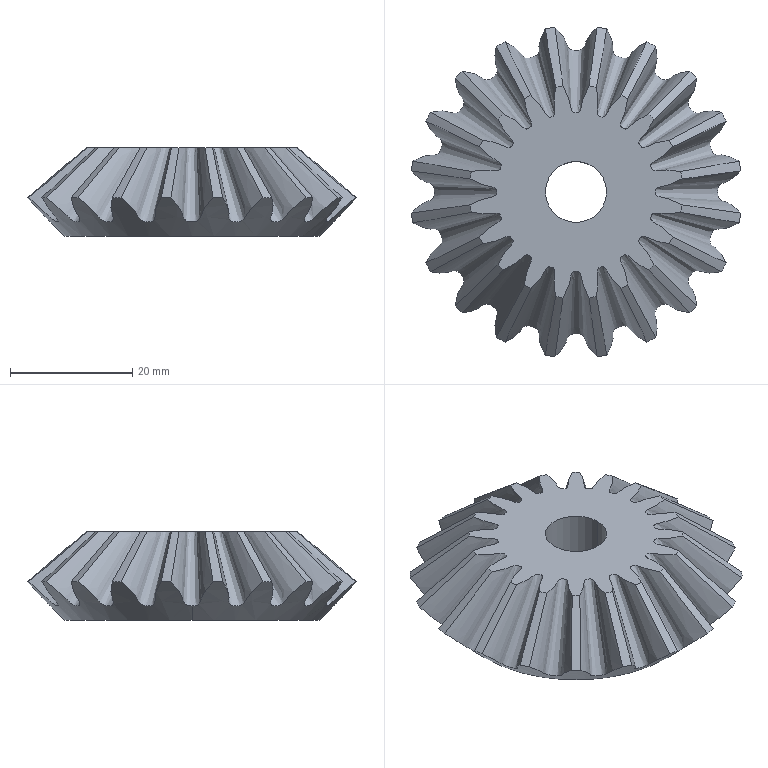Part | STEP file | Cuon T phu H01_12_Bevel01 | 1 solid | 46 faces | box 53.951 x 53.951 x 14.57 mm | volume 19453 mm3 | cone 22 | spline 20 | cylinder 2 | plane 2 | commonest cylinder face diameters 10 x2